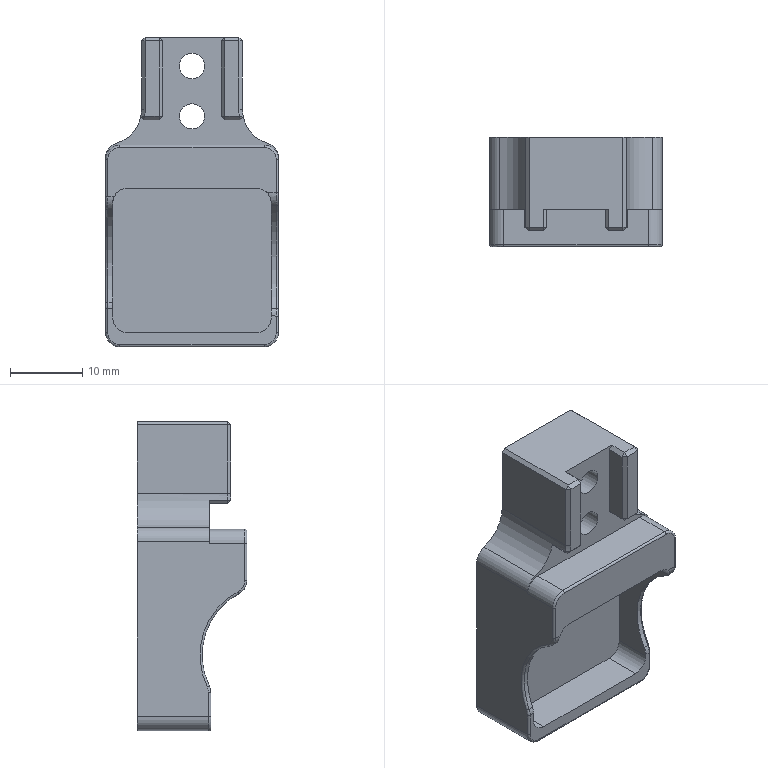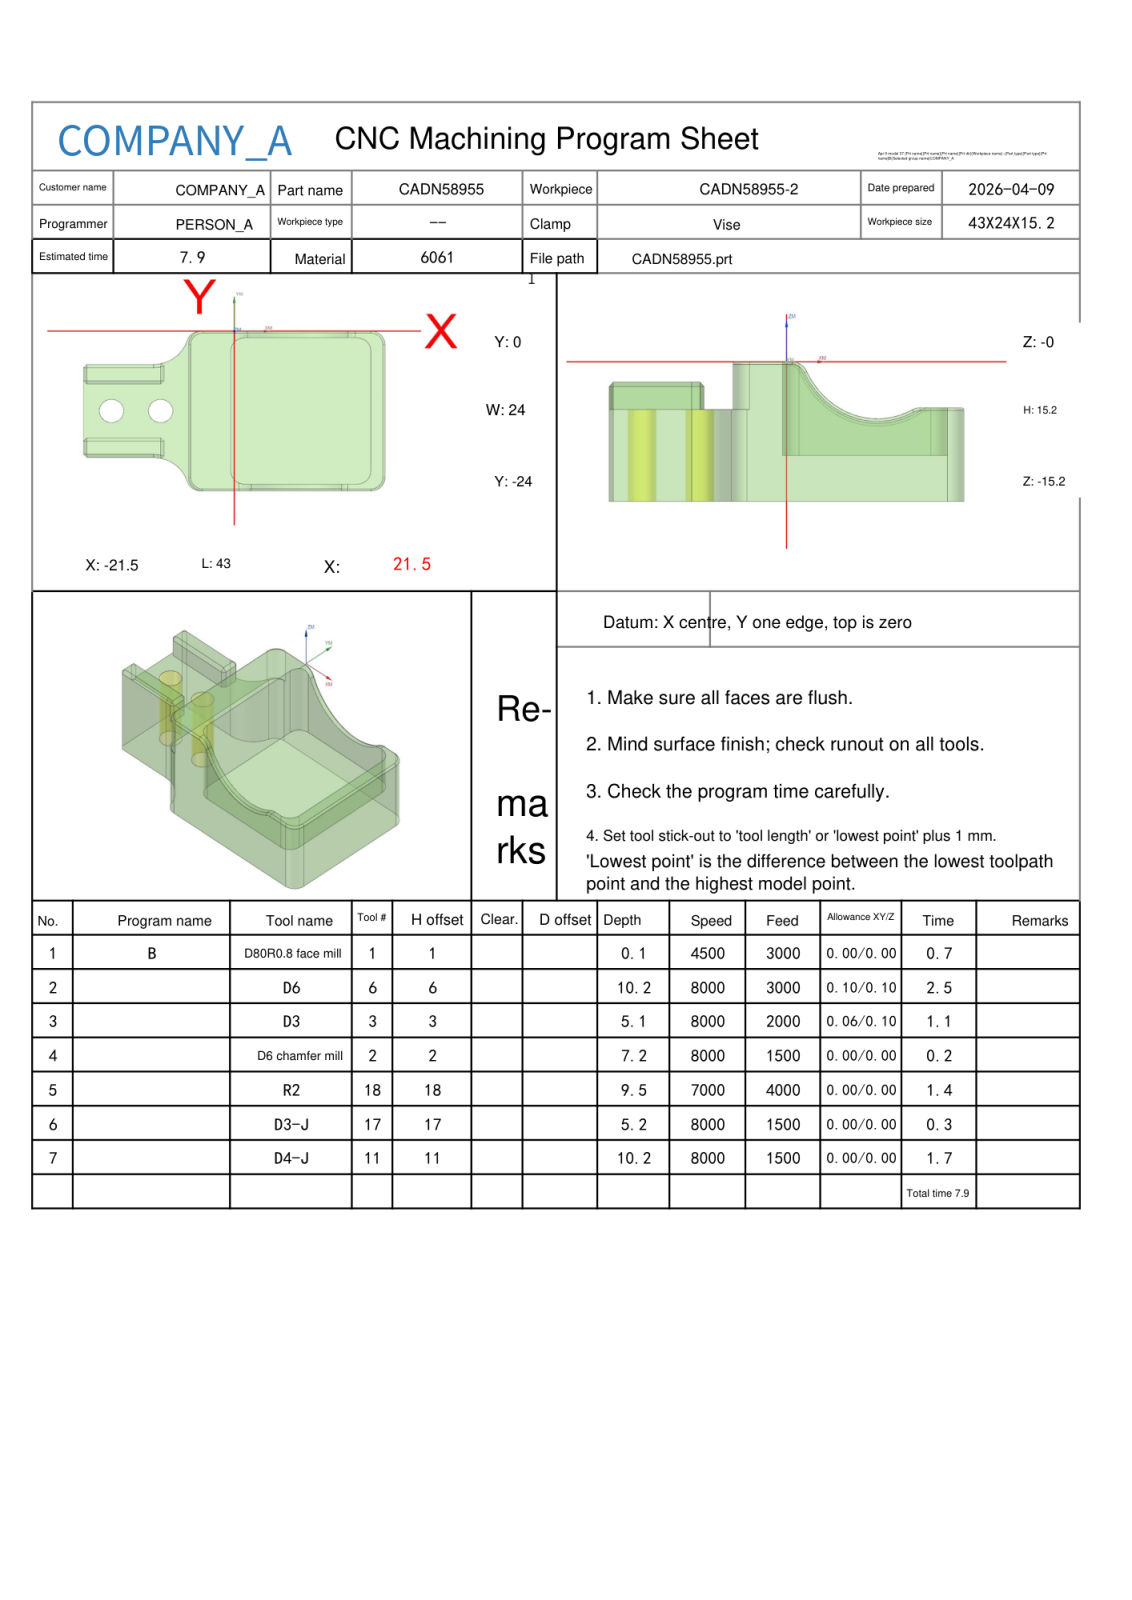NC program | NX | posted by the shop | part box 24 x 15.2 x 43 mm
Lines 10876 to 11083 of 14472:
N6 T17 M06
(D3-J  D=3. R=0. H=17 ce=0.40 di=0.00)
G00 G90 G54 X-9.471 Y-21.914 M03 S8000
G43 H17 Z14.5
M08
Z-3.7
G01 Z-5.2 F800.
X-8.538 Y-20.733
G03 X-8.473 Y-20.547 I-.235 J.186
X-8.587 Y-20.311 I-.3 J0.0
G01 X-8.629 Y-20.279
X-8.675 Y-20.184
X-8.631 Y-20.091
X-8.546 Y-20.022
X-8.49 Y-20.003
X-8.4 Y-20.092
Y-20.274
X-8.49 Y-20.364
X-8.546 Y-20.344
X-8.587 Y-20.311
X-8.629 Y-20.279
X-8.675 Y-20.184
X-8.631 Y-20.091
X-8.546 Y-20.022
X-8.49 Y-20.003
X-8.4 Y-20.092
Y-20.274
X-8.49 Y-20.364
X-8.546 Y-20.344
X-8.575 Y-20.321
G03 X-8.762 Y-20.256 I-.187 J-.235
G01 X-8.796 Y-20.258
X-9.701 Y-21.725
Z-3.7
G00 Z14.5
X-23.6 Y-12.6
Z-3.7
G01 Z-5.2
X-22.4
G03 X-21.8 Y-12. I0.0 J.6
G01 Y-10.119
G02 X-21.531 Y-9.85 I.27 J-.001
G01 X-9.713
X-8.728 Y-8.865
X-8.502 Y-8.639
X-8.46 Y-8.612
X-8.411 Y-8.632
X-8.4 Y-8.681
Y-15.319
X-8.411 Y-15.368
X-8.46 Y-15.388
X-8.502 Y-15.361
X-9.713 Y-14.15
X-21.531
G02 X-21.8 Y-13.881 I.001 J.27
G01 Y-10.5
G02 X-21.5 Y-10.2 I.3 J0.0
G01 X-21.342 Y-10.245
X-19.623 Y-11.305
X-19.577 Y-11.339
X-19.522 Y-11.355
X-19.466 Y-11.35
X-10.199
G02 X-9.9 Y-11.649 I-.001 J-.3
G01 Y-12.351
G02 X-10.199 Y-12.65 I-.3 J.001
G01 X-20.001
G02 X-20.3 Y-12.351 I.001 J.3
G01 Y-11.649
X-20.304 Y-11.591
X-20.288 Y-11.535
X-20.253 Y-11.488
G02 X-20.001 Y-11.35 I.253 J-.162
G01 X-19.301
G03 X-18.701 Y-10.75 I0.0 J.6
G01 Z-3.7
G00 Z14.5
X-9.701 Y-2.275
Z-3.7
G01 Z-5.2
X-8.808 Y-3.751
X-8.773 Y-3.753
G03 X-8.587 Y-3.689 I0.0 J.3
G01 X-8.546 Y-3.656
X-8.49 Y-3.636
X-8.4 Y-3.726
Y-3.908
X-8.49 Y-3.997
X-8.546 Y-3.978
X-8.631 Y-3.909
X-8.675 Y-3.816
X-8.629 Y-3.721
X-8.587 Y-3.689
X-8.546 Y-3.656
X-8.49 Y-3.636
X-8.4 Y-3.726
Y-3.908
X-8.49 Y-3.997
X-8.546 Y-3.978
X-8.631 Y-3.909
X-8.675 Y-3.816
X-8.629 Y-3.721
X-8.6 Y-3.699
G03 X-8.485 Y-3.463 I-.185 J.236
G01 X-8.549 Y-3.277
X-9.479 Y-2.092
Z-3.7
G00 Z14.5
G00 G90 X-15.121 Y-20.6 M03 S7000
Z14.5
Z-.7
G01 Z-2.2 F1500.
Y-19.4
G03 X-15.721 Y-18.8 I-.6 J0.0
G01 X-21.
G02 X-21.3 Y-18.5 I0.0 J.3
G01 Y-16.55
G02 X-21. Y-16.25 I.3 J0.0
G01 X-10.5
G02 X-10.2 Y-16.55 I0.0 J-.3
G01 Y-18.7
G02 X-10.41 Y-18.91 I-.21 J0.0
G01 X-10.448 Y-18.906
X-10.555 Y-18.887
G03 X-11.5 Y-18.8 I-.945 J-5.113
G01 X-15.721
X-16.721
G03 X-17.321 Y-19.4 I0.0 J-.6
G01 Y-20.6
Z-.7
G00 Z1.8
X-15.15 Y-9.55
Z-.7
G01 Z-2.2
Y-8.35
G03 X-15.75 Y-7.75 I-.6 J0.0
G01 X-21.
G02 X-21.3 Y-7.45 I0.0 J.3
G01 Y-5.5
G02 X-21. Y-5.2 I.3 J0.0
G01 X-11.5
G03 X-10.555 Y-5.113 I0.0 J5.2
G01 X-10.448 Y-5.094
X-10.41 Y-5.09
G02 X-10.2 Y-5.3 I0.0 J-.21
G01 Y-7.45
G02 X-10.5 Y-7.75 I-.3 J0.0
G01 X-15.75
X-16.75
G03 X-17.35 Y-8.35 I0.0 J-.6
G01 Y-9.55
Z-.7
G00 Z14.5
G00 G90 X-23.791 Y-16.02 M03 S8000
Z14.5
Z-4.2
G01 Z-5.2 F800.
G41 D17
X-23.6 Y-16.078
X-23.424 Y-16.104
G03 X-23. Y-15.929 I0.0 J.6
G01 X-21.621 Y-14.55
X-9.879
X-8.5 Y-15.929
Y-19.471
X-10.124 Y-20.782
G03 X-10.347 Y-21.249 I.377 J-.467
G01 X-10.346 Y-21.282
G40 X-10.335 Y-21.482
Z-4.2
G00 Z14.5
X-4.071 Y-26.3
Z-4.2
G01 Z-5.2
G41 D17
X-4.07 Y-26.1
Y-26.096
G03 X-4.645 Y-25.497 I-.6 J0.0
G02 X-8. Y-22. I.145 J3.497
G01 Y-2.
G02 X-4.645 Y1.497 I3.5 J0.0
G03 X-4.07 Y2.096 I-.025 J.599
G01 Y2.1
G40 X-4.071 Y2.3
Z-4.2
G00 Z14.5
X-10.335 Y-2.518
Z-4.2
G01 Z-5.2
G41 D17
X-10.346 Y-2.718
X-10.347 Y-2.751
G03 X-10.124 Y-3.218 I.6 J0.0
G01 X-8.5 Y-4.529
Y-8.071
X-9.879 Y-9.45
X-21.621
X-23. Y-8.071
G03 X-23.424 Y-7.896 I-.424 J-.424
G01 X-23.6 Y-7.922
G40 X-23.791 Y-7.98
Z-4.2
G00 Z14.5
G91 G28 Z0.0
M05
M09
G91 G28 Z0.0
M01